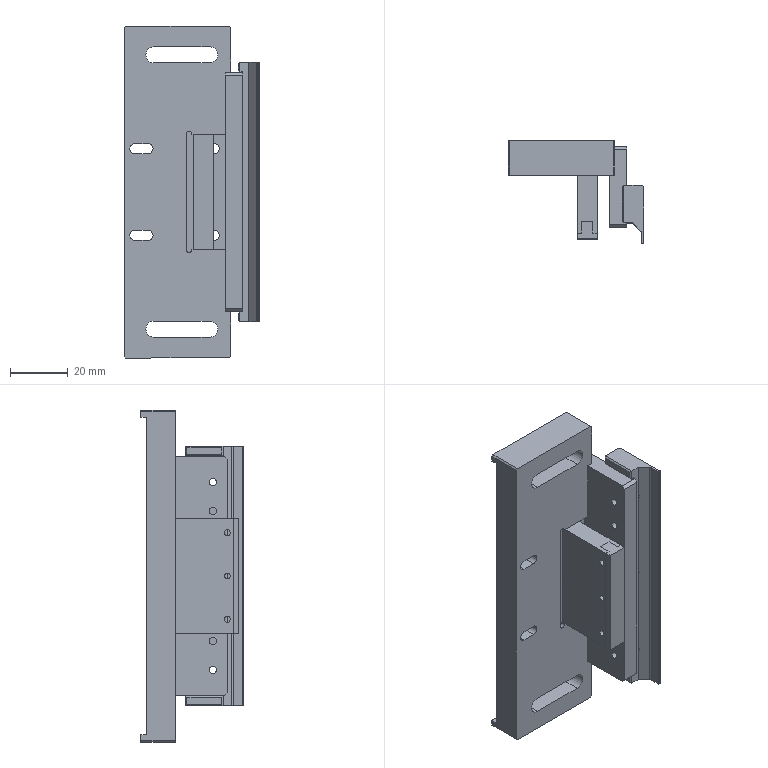Part | SolidWorks | 5 solids | 219 faces | box 47 x 35.487 x 115 mm | volume 62999 mm3 | plane 113 | cylinder 94 | cone 12 | commonest cylinder face diameters 2 x22 3.4 x18 6.5 x18 2.5 x16 3.3 x6 4.5 x6